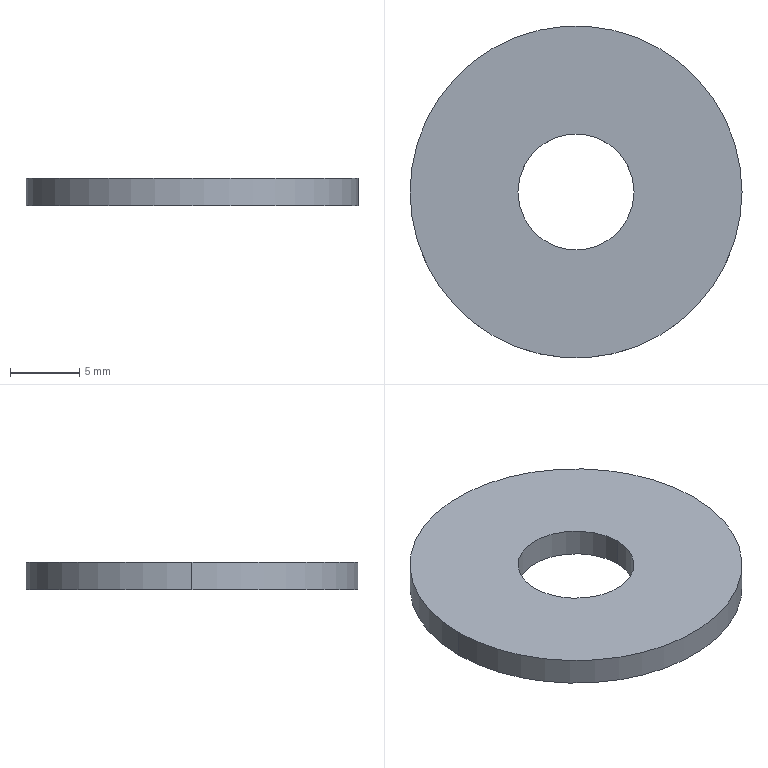Part | STEP file | PN_0014_Default<As Machined> | 1 solid | 6 faces | box 24 x 24 x 2 mm | volume 793.943 mm3 | cylinder 4 | plane 2 | commonest cylinder face diameters 8.4 x2 24 x2
STEP:
#1=CARTESIAN_POINT('',(-4.2,0.,-2.));
#2=VERTEX_POINT('',#1);
#3=CARTESIAN_POINT('',(4.2,0.,-2.));
#4=VERTEX_POINT('',#3);
#5=CARTESIAN_POINT('',(0.,0.,-2.));
#6=DIRECTION('',(0.,0.,1.));
#7=AXIS2_PLACEMENT_3D('',#5,#6,$);
#8=CIRCLE('',#7,4.2);
#9=EDGE_CURVE('',#2,#4,#8,.T.);
#10=ORIENTED_EDGE('',*,*,#9,.F.);
#11=CARTESIAN_POINT('',(-4.2,0.,0.));
#12=VERTEX_POINT('',#11);
#13=CARTESIAN_POINT('',(-4.2,0.,-2.));
#14=DIRECTION('',(0.,0.,1.));
#15=VECTOR('',#14,1.);
#16=LINE('',#13,#15);
#17=EDGE_CURVE('',#2,#12,#16,.T.);
#18=ORIENTED_EDGE('',*,*,#17,.T.);
#19=CARTESIAN_POINT('',(4.2,0.,0.));
#20=VERTEX_POINT('',#19);
#21=CARTESIAN_POINT('',(0.,0.,0.));
#22=DIRECTION('',(0.,0.,1.));
#23=AXIS2_PLACEMENT_3D('',#21,#22,$);
#24=CIRCLE('',#23,4.2);
#25=EDGE_CURVE('',#12,#20,#24,.T.);
#26=ORIENTED_EDGE('',*,*,#25,.T.);
#27=CARTESIAN_POINT('',(4.2,0.,-2.));
#28=DIRECTION('',(0.,0.,1.));
#29=VECTOR('',#28,1.);
#30=LINE('',#27,#29);
#31=EDGE_CURVE('',#4,#20,#30,.T.);
#32=ORIENTED_EDGE('',*,*,#31,.F.);
#33=EDGE_LOOP('',(#10,#18,#26,#32));
#34=FACE_OUTER_BOUND('',#33,.T.);
#35=CARTESIAN_POINT('',(0.,0.,-2.));
#36=DIRECTION('',(0.,0.,1.));
#37=DIRECTION('',(-1.,0.,0.));
#38=AXIS2_PLACEMENT_3D('',#35,#36,#37);
#39=CYLINDRICAL_SURFACE('',#38,4.2);
#40=ADVANCED_FACE('',(#34),#39,.F.);
#41=CARTESIAN_POINT('',(12.,0.,-2.));
#42=VERTEX_POINT('',#41);
#43=CARTESIAN_POINT('',(-12.,0.,-2.));
#44=VERTEX_POINT('',#43);
#45=CARTESIAN_POINT('',(0.,0.,-2.));
#46=DIRECTION('',(0.,0.,1.));
#47=AXIS2_PLACEMENT_3D('',#45,#46,$);
#48=CIRCLE('',#47,12.);
#49=EDGE_CURVE('',#42,#44,#48,.T.);
#50=ORIENTED_EDGE('',*,*,#49,.F.);
#51=CARTESIAN_POINT('',(0.,0.,-2.));
#52=DIRECTION('',(0.,0.,1.));
#53=AXIS2_PLACEMENT_3D('',#51,#52,$);
#54=CIRCLE('',#53,12.);
#55=EDGE_CURVE('',#44,#42,#54,.T.);
#56=ORIENTED_EDGE('',*,*,#55,.F.);
#57=EDGE_LOOP('',(#50,#56));
#58=FACE_OUTER_BOUND('',#57,.T.);
#59=CARTESIAN_POINT('',(0.,0.,-2.));
#60=DIRECTION('',(0.,0.,1.));
#61=AXIS2_PLACEMENT_3D('',#59,#60,$);
#62=CIRCLE('',#61,4.2);
#63=EDGE_CURVE('',#4,#2,#62,.T.);
#64=ORIENTED_EDGE('',*,*,#63,.T.);
#65=ORIENTED_EDGE('',*,*,#9,.T.);
#66=EDGE_LOOP('',(#64,#65));
#67=FACE_BOUND('',#66,.T.);
#68=CARTESIAN_POINT('',(0.,0.,-2.));
#69=DIRECTION('',(0.,0.,1.));
#70=DIRECTION('',(1.,0.,0.));
#71=AXIS2_PLACEMENT_3D('',#68,#69,#70);
#72=PLANE('',#71);
#73=ADVANCED_FACE('',(#58,#67),#72,.F.);
#74=ORIENTED_EDGE('',*,*,#17,.F.);
#75=ORIENTED_EDGE('',*,*,#63,.F.);
#76=ORIENTED_EDGE('',*,*,#31,.T.);
#77=CARTESIAN_POINT('',(0.,0.,0.));
#78=DIRECTION('',(0.,0.,1.));
#79=AXIS2_PLACEMENT_3D('',#77,#78,$);
#80=CIRCLE('',#79,4.2);
#81=EDGE_CURVE('',#20,#12,#80,.T.);
#82=ORIENTED_EDGE('',*,*,#81,.T.);
#83=EDGE_LOOP('',(#74,#75,#76,#82));
#84=FACE_OUTER_BOUND('',#83,.T.);
#85=CARTESIAN_POINT('',(0.,0.,-2.));
#86=DIRECTION('',(0.,0.,1.));
#87=DIRECTION('',(1.,0.,0.));
#88=AXIS2_PLACEMENT_3D('',#85,#86,#87);
#89=CYLINDRICAL_SURFACE('',#88,4.2);
#90=ADVANCED_FACE('',(#84),#89,.F.);
#91=CARTESIAN_POINT('',(12.,0.,0.));
#92=VERTEX_POINT('',#91);
#93=CARTESIAN_POINT('',(-12.,0.,0.));
#94=VERTEX_POINT('',#93);
#95=CARTESIAN_POINT('',(0.,0.,0.));
#96=DIRECTION('',(0.,0.,1.));
#97=AXIS2_PLACEMENT_3D('',#95,#96,$);
#98=CIRCLE('',#97,12.);
#99=EDGE_CURVE('',#92,#94,#98,.T.);
#100=ORIENTED_EDGE('',*,*,#99,.T.);
#101=CARTESIAN_POINT('',(0.,0.,0.));
#102=DIRECTION('',(0.,0.,1.));
#103=AXIS2_PLACEMENT_3D('',#101,#102,$);
#104=CIRCLE('',#103,12.);
#105=EDGE_CURVE('',#94,#92,#104,.T.);
#106=ORIENTED_EDGE('',*,*,#105,.T.);
#107=EDGE_LOOP('',(#100,#106));
#108=FACE_OUTER_BOUND('',#107,.T.);
#109=ORIENTED_EDGE('',*,*,#81,.F.);
#110=ORIENTED_EDGE('',*,*,#25,.F.);
#111=EDGE_LOOP('',(#109,#110));
#112=FACE_BOUND('',#111,.T.);
#113=CARTESIAN_POINT('',(0.,0.,0.));
#114=DIRECTION('',(0.,0.,1.));
#115=DIRECTION('',(1.,0.,0.));
#116=AXIS2_PLACEMENT_3D('',#113,#114,#115);
#117=PLANE('',#116);
#118=ADVANCED_FACE('',(#108,#112),#117,.T.);
#119=ORIENTED_EDGE('',*,*,#49,.T.);
#120=CARTESIAN_POINT('',(-12.,0.,-2.));
#121=DIRECTION('',(0.,0.,1.));
#122=VECTOR('',#121,1.);
#123=LINE('',#120,#122);
#124=EDGE_CURVE('',#44,#94,#123,.T.);
#125=ORIENTED_EDGE('',*,*,#124,.T.);
#126=ORIENTED_EDGE('',*,*,#99,.F.);
#127=CARTESIAN_POINT('',(12.,0.,-2.));
#128=DIRECTION('',(0.,0.,1.));
#129=VECTOR('',#128,1.);
#130=LINE('',#127,#129);
#131=EDGE_CURVE('',#42,#92,#130,.T.);
#132=ORIENTED_EDGE('',*,*,#131,.F.);
#133=EDGE_LOOP('',(#119,#125,#126,#132));
#134=FACE_OUTER_BOUND('',#133,.T.);
#135=CARTESIAN_POINT('',(0.,0.,-2.));
#136=DIRECTION('',(0.,0.,1.));
#137=DIRECTION('',(1.,0.,0.));
#138=AXIS2_PLACEMENT_3D('',#135,#136,#137);
#139=CYLINDRICAL_SURFACE('',#138,12.);
#140=ADVANCED_FACE('',(#134),#139,.T.);
#141=ORIENTED_EDGE('',*,*,#124,.F.);
#142=ORIENTED_EDGE('',*,*,#55,.T.);
#143=ORIENTED_EDGE('',*,*,#131,.T.);
#144=ORIENTED_EDGE('',*,*,#105,.F.);
#145=EDGE_LOOP('',(#141,#142,#143,#144));
#146=FACE_OUTER_BOUND('',#145,.T.);
#147=CARTESIAN_POINT('',(0.,0.,-2.));
#148=DIRECTION('',(0.,0.,1.));
#149=DIRECTION('',(-1.,0.,0.));
#150=AXIS2_PLACEMENT_3D('',#147,#148,#149);
#151=CYLINDRICAL_SURFACE('',#150,12.);
#152=ADVANCED_FACE('',(#146),#151,.T.);
#153=CLOSED_SHELL('',(#40,#73,#90,#118,#140,#152));
#154=MANIFOLD_SOLID_BREP('',#153);
#155=(LENGTH_UNIT()NAMED_UNIT(*)SI_UNIT(.MILLI.,.METRE.));
#156=UNCERTAINTY_MEASURE_WITH_UNIT(LENGTH_MEASURE(0.005),#155,'','');
#157=(NAMED_UNIT(*)PLANE_ANGLE_UNIT()SI_UNIT($,.RADIAN.));
#158=(NAMED_UNIT(*)SI_UNIT($,.STERADIAN.)SOLID_ANGLE_UNIT());
#159=(GEOMETRIC_REPRESENTATION_CONTEXT(3)GLOBAL_UNCERTAINTY_ASSIGNED_CONTEXT((#156))GLOBAL_UNIT_ASSIGNED_CONTEXT((#155,#157,#158))REPRESENTATION_CONTEXT('',''));
#160=ADVANCED_BREP_SHAPE_REPRESENTATION('',(#154),#159);